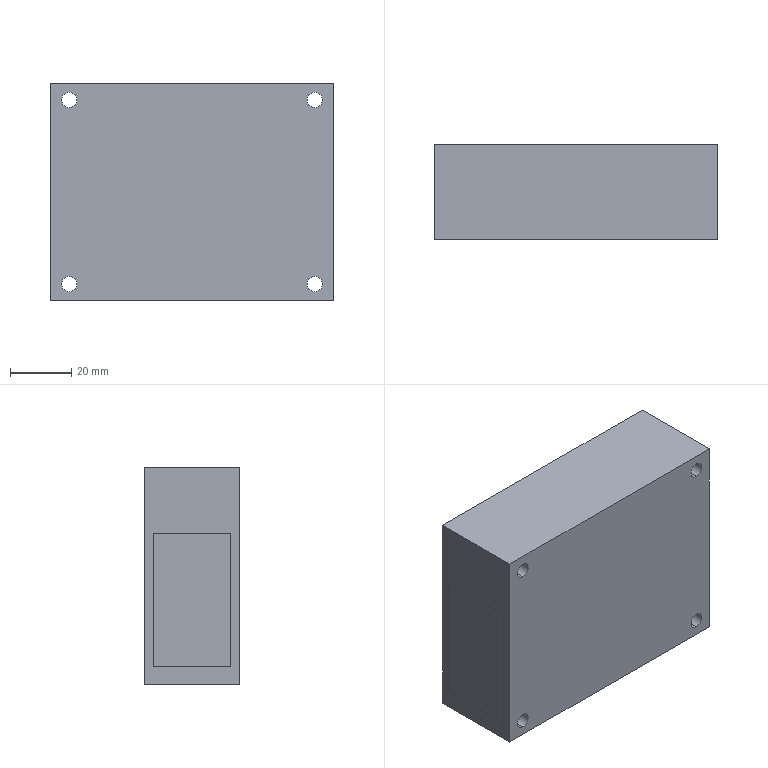Part | STEP file | Laser ranging sensor 1200mm | 1 solid | 19 faces | box 92 x 31 x 71 mm | volume 199839 mm3 | plane 11 | cylinder 8 | commonest cylinder face diameters 5 x8
STEP:
#1=CARTESIAN_POINT('',(-40.,15.5,-32.5));
#2=VERTEX_POINT('',#1);
#3=CARTESIAN_POINT('',(-40.,15.5,-27.5));
#4=VERTEX_POINT('',#3);
#5=CARTESIAN_POINT('',(-40.,15.5,-30.));
#6=DIRECTION('',(0.,1.,0.));
#7=DIRECTION('',(0.,0.,1.));
#8=AXIS2_PLACEMENT_3D('',#5,#6,#7);
#9=CIRCLE('',#8,2.5);
#10=EDGE_CURVE('',#2,#4,#9,.T.);
#11=ORIENTED_EDGE('',*,*,#10,.T.);
#12=CARTESIAN_POINT('',(-40.,-15.5,-27.5));
#13=VERTEX_POINT('',#12);
#14=CARTESIAN_POINT('',(-40.,15.5,-27.5));
#15=DIRECTION('',(0.,-1.,0.));
#16=VECTOR('',#15,1000.);
#17=LINE('',#14,#16);
#18=EDGE_CURVE('',#4,#13,#17,.T.);
#19=ORIENTED_EDGE('',*,*,#18,.T.);
#20=CARTESIAN_POINT('',(-40.,-15.5,-32.5));
#21=VERTEX_POINT('',#20);
#22=CARTESIAN_POINT('',(-40.,-15.5,-30.));
#23=DIRECTION('',(0.,1.,0.));
#24=DIRECTION('',(0.,0.,1.));
#25=AXIS2_PLACEMENT_3D('',#22,#23,#24);
#26=CIRCLE('',#25,2.5);
#27=EDGE_CURVE('',#21,#13,#26,.T.);
#28=ORIENTED_EDGE('',*,*,#27,.F.);
#29=CARTESIAN_POINT('',(-40.,15.5,-32.5));
#30=DIRECTION('',(0.,-1.,0.));
#31=VECTOR('',#30,1000.);
#32=LINE('',#29,#31);
#33=EDGE_CURVE('',#2,#21,#32,.T.);
#34=ORIENTED_EDGE('',*,*,#33,.F.);
#35=EDGE_LOOP('',(#11,#19,#28,#34));
#36=FACE_OUTER_BOUND('',#35,.T.);
#37=CARTESIAN_POINT('',(-40.,15.5,-30.));
#38=DIRECTION('',(0.,-1.,0.));
#39=DIRECTION('',(0.,0.,-1.));
#40=AXIS2_PLACEMENT_3D('',#37,#38,#39);
#41=CYLINDRICAL_SURFACE('',#40,2.5);
#42=ADVANCED_FACE('',(#36),#41,.F.);
#43=CARTESIAN_POINT('',(40.,15.5,-32.5));
#44=VERTEX_POINT('',#43);
#45=CARTESIAN_POINT('',(40.,15.5,-27.5));
#46=VERTEX_POINT('',#45);
#47=CARTESIAN_POINT('',(40.,15.5,-30.));
#48=DIRECTION('',(0.,1.,0.));
#49=DIRECTION('',(0.,0.,1.));
#50=AXIS2_PLACEMENT_3D('',#47,#48,#49);
#51=CIRCLE('',#50,2.5);
#52=EDGE_CURVE('',#44,#46,#51,.T.);
#53=ORIENTED_EDGE('',*,*,#52,.T.);
#54=CARTESIAN_POINT('',(40.,-15.5,-27.5));
#55=VERTEX_POINT('',#54);
#56=CARTESIAN_POINT('',(40.,15.5,-27.5));
#57=DIRECTION('',(0.,-1.,0.));
#58=VECTOR('',#57,1000.);
#59=LINE('',#56,#58);
#60=EDGE_CURVE('',#46,#55,#59,.T.);
#61=ORIENTED_EDGE('',*,*,#60,.T.);
#62=CARTESIAN_POINT('',(40.,-15.5,-32.5));
#63=VERTEX_POINT('',#62);
#64=CARTESIAN_POINT('',(40.,-15.5,-30.));
#65=DIRECTION('',(0.,1.,0.));
#66=DIRECTION('',(0.,0.,1.));
#67=AXIS2_PLACEMENT_3D('',#64,#65,#66);
#68=CIRCLE('',#67,2.5);
#69=EDGE_CURVE('',#63,#55,#68,.T.);
#70=ORIENTED_EDGE('',*,*,#69,.F.);
#71=CARTESIAN_POINT('',(40.,15.5,-32.5));
#72=DIRECTION('',(0.,-1.,0.));
#73=VECTOR('',#72,1000.);
#74=LINE('',#71,#73);
#75=EDGE_CURVE('',#44,#63,#74,.T.);
#76=ORIENTED_EDGE('',*,*,#75,.F.);
#77=EDGE_LOOP('',(#53,#61,#70,#76));
#78=FACE_OUTER_BOUND('',#77,.T.);
#79=CARTESIAN_POINT('',(40.,15.5,-30.));
#80=DIRECTION('',(0.,-1.,0.));
#81=DIRECTION('',(0.,0.,-1.));
#82=AXIS2_PLACEMENT_3D('',#79,#80,#81);
#83=CYLINDRICAL_SURFACE('',#82,2.5);
#84=ADVANCED_FACE('',(#78),#83,.F.);
#85=CARTESIAN_POINT('',(40.,15.5,27.5));
#86=VERTEX_POINT('',#85);
#87=CARTESIAN_POINT('',(40.,15.5,32.5));
#88=VERTEX_POINT('',#87);
#89=CARTESIAN_POINT('',(40.,15.5,30.));
#90=DIRECTION('',(0.,1.,0.));
#91=DIRECTION('',(0.,0.,1.));
#92=AXIS2_PLACEMENT_3D('',#89,#90,#91);
#93=CIRCLE('',#92,2.5);
#94=EDGE_CURVE('',#86,#88,#93,.T.);
#95=ORIENTED_EDGE('',*,*,#94,.T.);
#96=CARTESIAN_POINT('',(40.,-15.5,32.5));
#97=VERTEX_POINT('',#96);
#98=CARTESIAN_POINT('',(40.,15.5,32.5));
#99=DIRECTION('',(0.,-1.,0.));
#100=VECTOR('',#99,1000.);
#101=LINE('',#98,#100);
#102=EDGE_CURVE('',#88,#97,#101,.T.);
#103=ORIENTED_EDGE('',*,*,#102,.T.);
#104=CARTESIAN_POINT('',(40.,-15.5,27.5));
#105=VERTEX_POINT('',#104);
#106=CARTESIAN_POINT('',(40.,-15.5,30.));
#107=DIRECTION('',(0.,1.,0.));
#108=DIRECTION('',(0.,0.,1.));
#109=AXIS2_PLACEMENT_3D('',#106,#107,#108);
#110=CIRCLE('',#109,2.5);
#111=EDGE_CURVE('',#105,#97,#110,.T.);
#112=ORIENTED_EDGE('',*,*,#111,.F.);
#113=CARTESIAN_POINT('',(40.,15.5,27.5));
#114=DIRECTION('',(0.,-1.,0.));
#115=VECTOR('',#114,1000.);
#116=LINE('',#113,#115);
#117=EDGE_CURVE('',#86,#105,#116,.T.);
#118=ORIENTED_EDGE('',*,*,#117,.F.);
#119=EDGE_LOOP('',(#95,#103,#112,#118));
#120=FACE_OUTER_BOUND('',#119,.T.);
#121=CARTESIAN_POINT('',(40.,15.5,30.));
#122=DIRECTION('',(0.,-1.,0.));
#123=DIRECTION('',(0.,0.,-1.));
#124=AXIS2_PLACEMENT_3D('',#121,#122,#123);
#125=CYLINDRICAL_SURFACE('',#124,2.5);
#126=ADVANCED_FACE('',(#120),#125,.F.);
#127=CARTESIAN_POINT('',(-40.,15.5,27.5));
#128=VERTEX_POINT('',#127);
#129=CARTESIAN_POINT('',(-40.,15.5,32.5));
#130=VERTEX_POINT('',#129);
#131=CARTESIAN_POINT('',(-40.,15.5,30.));
#132=DIRECTION('',(0.,1.,0.));
#133=DIRECTION('',(0.,0.,1.));
#134=AXIS2_PLACEMENT_3D('',#131,#132,#133);
#135=CIRCLE('',#134,2.5);
#136=EDGE_CURVE('',#128,#130,#135,.T.);
#137=ORIENTED_EDGE('',*,*,#136,.T.);
#138=CARTESIAN_POINT('',(-40.,-15.5,32.5));
#139=VERTEX_POINT('',#138);
#140=CARTESIAN_POINT('',(-40.,15.5,32.5));
#141=DIRECTION('',(0.,-1.,0.));
#142=VECTOR('',#141,1000.);
#143=LINE('',#140,#142);
#144=EDGE_CURVE('',#130,#139,#143,.T.);
#145=ORIENTED_EDGE('',*,*,#144,.T.);
#146=CARTESIAN_POINT('',(-40.,-15.5,27.5));
#147=VERTEX_POINT('',#146);
#148=CARTESIAN_POINT('',(-40.,-15.5,30.));
#149=DIRECTION('',(0.,1.,0.));
#150=DIRECTION('',(0.,0.,1.));
#151=AXIS2_PLACEMENT_3D('',#148,#149,#150);
#152=CIRCLE('',#151,2.5);
#153=EDGE_CURVE('',#147,#139,#152,.T.);
#154=ORIENTED_EDGE('',*,*,#153,.F.);
#155=CARTESIAN_POINT('',(-40.,15.5,27.5));
#156=DIRECTION('',(0.,-1.,0.));
#157=VECTOR('',#156,1000.);
#158=LINE('',#155,#157);
#159=EDGE_CURVE('',#128,#147,#158,.T.);
#160=ORIENTED_EDGE('',*,*,#159,.F.);
#161=EDGE_LOOP('',(#137,#145,#154,#160));
#162=FACE_OUTER_BOUND('',#161,.T.);
#163=CARTESIAN_POINT('',(-40.,15.5,30.));
#164=DIRECTION('',(0.,-1.,0.));
#165=DIRECTION('',(0.,0.,-1.));
#166=AXIS2_PLACEMENT_3D('',#163,#164,#165);
#167=CYLINDRICAL_SURFACE('',#166,2.5);
#168=ADVANCED_FACE('',(#162),#167,.F.);
#169=CARTESIAN_POINT('',(46.,15.5,35.5));
#170=VERTEX_POINT('',#169);
#171=CARTESIAN_POINT('',(46.,15.5,-35.5));
#172=VERTEX_POINT('',#171);
#173=CARTESIAN_POINT('',(46.,15.5,35.5));
#174=DIRECTION('',(0.,0.,-1.));
#175=VECTOR('',#174,1000.);
#176=LINE('',#173,#175);
#177=EDGE_CURVE('',#170,#172,#176,.T.);
#178=ORIENTED_EDGE('',*,*,#177,.T.);
#179=CARTESIAN_POINT('',(-46.,15.5,-35.5));
#180=VERTEX_POINT('',#179);
#181=CARTESIAN_POINT('',(-46.,15.5,-35.5));
#182=DIRECTION('',(-1.,0.,0.));
#183=VECTOR('',#182,1000.);
#184=LINE('',#181,#183);
#185=EDGE_CURVE('',#172,#180,#184,.T.);
#186=ORIENTED_EDGE('',*,*,#185,.T.);
#187=CARTESIAN_POINT('',(-46.,15.5,35.5));
#188=VERTEX_POINT('',#187);
#189=CARTESIAN_POINT('',(-46.,15.5,35.5));
#190=DIRECTION('',(0.,0.,1.));
#191=VECTOR('',#190,1000.);
#192=LINE('',#189,#191);
#193=EDGE_CURVE('',#180,#188,#192,.T.);
#194=ORIENTED_EDGE('',*,*,#193,.T.);
#195=CARTESIAN_POINT('',(-46.,15.5,35.5));
#196=DIRECTION('',(1.,0.,0.));
#197=VECTOR('',#196,1000.);
#198=LINE('',#195,#197);
#199=EDGE_CURVE('',#188,#170,#198,.T.);
#200=ORIENTED_EDGE('',*,*,#199,.T.);
#201=EDGE_LOOP('',(#178,#186,#194,#200));
#202=FACE_OUTER_BOUND('',#201,.T.);
#203=ORIENTED_EDGE('',*,*,#136,.F.);
#204=CARTESIAN_POINT('',(-40.,15.5,30.));
#205=DIRECTION('',(0.,1.,0.));
#206=DIRECTION('',(0.,0.,1.));
#207=AXIS2_PLACEMENT_3D('',#204,#205,#206);
#208=CIRCLE('',#207,2.5);
#209=EDGE_CURVE('',#130,#128,#208,.T.);
#210=ORIENTED_EDGE('',*,*,#209,.F.);
#211=EDGE_LOOP('',(#203,#210));
#212=FACE_BOUND('',#211,.T.);
#213=ORIENTED_EDGE('',*,*,#94,.F.);
#214=CARTESIAN_POINT('',(40.,15.5,30.));
#215=DIRECTION('',(0.,1.,0.));
#216=DIRECTION('',(0.,0.,1.));
#217=AXIS2_PLACEMENT_3D('',#214,#215,#216);
#218=CIRCLE('',#217,2.5);
#219=EDGE_CURVE('',#88,#86,#218,.T.);
#220=ORIENTED_EDGE('',*,*,#219,.F.);
#221=EDGE_LOOP('',(#213,#220));
#222=FACE_BOUND('',#221,.T.);
#223=ORIENTED_EDGE('',*,*,#52,.F.);
#224=CARTESIAN_POINT('',(40.,15.5,-30.));
#225=DIRECTION('',(0.,1.,0.));
#226=DIRECTION('',(0.,0.,1.));
#227=AXIS2_PLACEMENT_3D('',#224,#225,#226);
#228=CIRCLE('',#227,2.5);
#229=EDGE_CURVE('',#46,#44,#228,.T.);
#230=ORIENTED_EDGE('',*,*,#229,.F.);
#231=EDGE_LOOP('',(#223,#230));
#232=FACE_BOUND('',#231,.T.);
#233=ORIENTED_EDGE('',*,*,#10,.F.);
#234=CARTESIAN_POINT('',(-40.,15.5,-30.));
#235=DIRECTION('',(0.,1.,0.));
#236=DIRECTION('',(0.,0.,1.));
#237=AXIS2_PLACEMENT_3D('',#234,#235,#236);
#238=CIRCLE('',#237,2.5);
#239=EDGE_CURVE('',#4,#2,#238,.T.);
#240=ORIENTED_EDGE('',*,*,#239,.F.);
#241=EDGE_LOOP('',(#233,#240));
#242=FACE_BOUND('',#241,.T.);
#243=CARTESIAN_POINT('',(0.,15.5,0.));
#244=DIRECTION('',(0.,-1.,0.));
#245=DIRECTION('',(0.,0.,-1.));
#246=AXIS2_PLACEMENT_3D('',#243,#244,#245);
#247=PLANE('',#246);
#248=ADVANCED_FACE('',(#202,#212,#222,#232,#242),#247,.F.);
#249=ORIENTED_EDGE('',*,*,#69,.T.);
#250=CARTESIAN_POINT('',(40.,-15.5,-30.));
#251=DIRECTION('',(0.,1.,0.));
#252=DIRECTION('',(0.,0.,1.));
#253=AXIS2_PLACEMENT_3D('',#250,#251,#252);
#254=CIRCLE('',#253,2.5);
#255=EDGE_CURVE('',#55,#63,#254,.T.);
#256=ORIENTED_EDGE('',*,*,#255,.T.);
#257=EDGE_LOOP('',(#249,#256));
#258=FACE_BOUND('',#257,.T.);
#259=ORIENTED_EDGE('',*,*,#153,.T.);
#260=CARTESIAN_POINT('',(-40.,-15.5,30.));
#261=DIRECTION('',(0.,1.,0.));
#262=DIRECTION('',(0.,0.,1.));
#263=AXIS2_PLACEMENT_3D('',#260,#261,#262);
#264=CIRCLE('',#263,2.5);
#265=EDGE_CURVE('',#139,#147,#264,.T.);
#266=ORIENTED_EDGE('',*,*,#265,.T.);
#267=EDGE_LOOP('',(#259,#266));
#268=FACE_BOUND('',#267,.T.);
#269=CARTESIAN_POINT('',(46.,-15.5,35.5));
#270=VERTEX_POINT('',#269);
#271=CARTESIAN_POINT('',(46.,-15.5,-35.5));
#272=VERTEX_POINT('',#271);
#273=CARTESIAN_POINT('',(46.,-15.5,35.5));
#274=DIRECTION('',(0.,0.,-1.));
#275=VECTOR('',#274,1000.);
#276=LINE('',#273,#275);
#277=EDGE_CURVE('',#270,#272,#276,.T.);
#278=ORIENTED_EDGE('',*,*,#277,.F.);
#279=CARTESIAN_POINT('',(-46.,-15.5,35.5));
#280=VERTEX_POINT('',#279);
#281=CARTESIAN_POINT('',(-46.,-15.5,35.5));
#282=DIRECTION('',(1.,0.,0.));
#283=VECTOR('',#282,1000.);
#284=LINE('',#281,#283);
#285=EDGE_CURVE('',#280,#270,#284,.T.);
#286=ORIENTED_EDGE('',*,*,#285,.F.);
#287=CARTESIAN_POINT('',(-46.,-15.5,-35.5));
#288=VERTEX_POINT('',#287);
#289=CARTESIAN_POINT('',(-46.,-15.5,35.5));
#290=DIRECTION('',(0.,0.,1.));
#291=VECTOR('',#290,1000.);
#292=LINE('',#289,#291);
#293=EDGE_CURVE('',#288,#280,#292,.T.);
#294=ORIENTED_EDGE('',*,*,#293,.F.);
#295=CARTESIAN_POINT('',(-46.,-15.5,-35.5));
#296=DIRECTION('',(-1.,0.,0.));
#297=VECTOR('',#296,1000.);
#298=LINE('',#295,#297);
#299=EDGE_CURVE('',#272,#288,#298,.T.);
#300=ORIENTED_EDGE('',*,*,#299,.F.);
#301=EDGE_LOOP('',(#278,#286,#294,#300));
#302=FACE_OUTER_BOUND('',#301,.T.);
#303=ORIENTED_EDGE('',*,*,#111,.T.);
#304=CARTESIAN_POINT('',(40.,-15.5,30.));
#305=DIRECTION('',(0.,1.,0.));
#306=DIRECTION('',(0.,0.,1.));
#307=AXIS2_PLACEMENT_3D('',#304,#305,#306);
#308=CIRCLE('',#307,2.5);
#309=EDGE_CURVE('',#97,#105,#308,.T.);
#310=ORIENTED_EDGE('',*,*,#309,.T.);
#311=EDGE_LOOP('',(#303,#310));
#312=FACE_BOUND('',#311,.T.);
#313=ORIENTED_EDGE('',*,*,#27,.T.);
#314=CARTESIAN_POINT('',(-40.,-15.5,-30.));
#315=DIRECTION('',(0.,1.,0.));
#316=DIRECTION('',(0.,0.,1.));
#317=AXIS2_PLACEMENT_3D('',#314,#315,#316);
#318=CIRCLE('',#317,2.5);
#319=EDGE_CURVE('',#13,#21,#318,.T.);
#320=ORIENTED_EDGE('',*,*,#319,.T.);
#321=EDGE_LOOP('',(#313,#320));
#322=FACE_BOUND('',#321,.T.);
#323=CARTESIAN_POINT('',(0.,-15.5,0.));
#324=DIRECTION('',(0.,-1.,0.));
#325=DIRECTION('',(0.,0.,-1.));
#326=AXIS2_PLACEMENT_3D('',#323,#324,#325);
#327=PLANE('',#326);
#328=ADVANCED_FACE('',(#258,#268,#302,#312,#322),#327,.T.);
#329=ORIENTED_EDGE('',*,*,#277,.T.);
#330=CARTESIAN_POINT('',(46.,15.5,-35.5));
#331=DIRECTION('',(0.,-1.,0.));
#332=VECTOR('',#331,1000.);
#333=LINE('',#330,#332);
#334=EDGE_CURVE('',#172,#272,#333,.T.);
#335=ORIENTED_EDGE('',*,*,#334,.F.);
#336=ORIENTED_EDGE('',*,*,#177,.F.);
#337=CARTESIAN_POINT('',(46.,15.5,35.5));
#338=DIRECTION('',(0.,-1.,0.));
#339=VECTOR('',#338,1000.);
#340=LINE('',#337,#339);
#341=EDGE_CURVE('',#170,#270,#340,.T.);
#342=ORIENTED_EDGE('',*,*,#341,.T.);
#343=EDGE_LOOP('',(#329,#335,#336,#342));
#344=FACE_OUTER_BOUND('',#343,.T.);
#345=CARTESIAN_POINT('',(46.,15.5,35.5));
#346=DIRECTION('',(-1.,0.,0.));
#347=DIRECTION('',(0.,0.,1.));
#348=AXIS2_PLACEMENT_3D('',#345,#346,#347);
#349=PLANE('',#348);
#350=ADVANCED_FACE('',(#344),#349,.F.);
#351=ORIENTED_EDGE('',*,*,#299,.T.);
#352=CARTESIAN_POINT('',(-46.,15.5,-35.5));
#353=DIRECTION('',(0.,-1.,0.));
#354=VECTOR('',#353,1000.);
#355=LINE('',#352,#354);
#356=EDGE_CURVE('',#180,#288,#355,.T.);
#357=ORIENTED_EDGE('',*,*,#356,.F.);
#358=ORIENTED_EDGE('',*,*,#185,.F.);
#359=ORIENTED_EDGE('',*,*,#334,.T.);
#360=EDGE_LOOP('',(#351,#357,#358,#359));
#361=FACE_OUTER_BOUND('',#360,.T.);
#362=CARTESIAN_POINT('',(-46.,15.5,-35.5));
#363=DIRECTION('',(0.,0.,1.));
#364=DIRECTION('',(1.,0.,0.));
#365=AXIS2_PLACEMENT_3D('',#362,#363,#364);
#366=PLANE('',#365);
#367=ADVANCED_FACE('',(#361),#366,.F.);
#368=CARTESIAN_POINT('',(-46.,12.595,13.805));
#369=VERTEX_POINT('',#368);
#370=CARTESIAN_POINT('',(-46.,12.595,-29.542));
#371=VERTEX_POINT('',#370);
#372=CARTESIAN_POINT('',(-46.,12.595,-29.542));
#373=DIRECTION('',(0.,0.,-1.));
#374=VECTOR('',#373,1000.);
#375=LINE('',#372,#374);
#376=EDGE_CURVE('',#369,#371,#375,.T.);
#377=ORIENTED_EDGE('',*,*,#376,.F.);
#378=CARTESIAN_POINT('',(-46.,-12.595,13.805));
#379=VERTEX_POINT('',#378);
#380=CARTESIAN_POINT('',(-46.,-12.595,13.805));
#381=DIRECTION('',(0.,1.,0.));
#382=VECTOR('',#381,1000.);
#383=LINE('',#380,#382);
#384=EDGE_CURVE('',#379,#369,#383,.T.);
#385=ORIENTED_EDGE('',*,*,#384,.F.);
#386=CARTESIAN_POINT('',(-46.,-12.595,-29.542));
#387=VERTEX_POINT('',#386);
#388=CARTESIAN_POINT('',(-46.,-12.595,-29.542));
#389=DIRECTION('',(0.,0.,1.));
#390=VECTOR('',#389,1000.);
#391=LINE('',#388,#390);
#392=EDGE_CURVE('',#387,#379,#391,.T.);
#393=ORIENTED_EDGE('',*,*,#392,.F.);
#394=CARTESIAN_POINT('',(-46.,-12.595,-29.542));
#395=DIRECTION('',(0.,-1.,0.));
#396=VECTOR('',#395,1000.);
#397=LINE('',#394,#396);
#398=EDGE_CURVE('',#371,#387,#397,.T.);
#399=ORIENTED_EDGE('',*,*,#398,.F.);
#400=EDGE_LOOP('',(#377,#385,#393,#399));
#401=FACE_BOUND('',#400,.T.);
#402=ORIENTED_EDGE('',*,*,#293,.T.);
#403=CARTESIAN_POINT('',(-46.,15.5,35.5));
#404=DIRECTION('',(0.,-1.,0.));
#405=VECTOR('',#404,1000.);
#406=LINE('',#403,#405);
#407=EDGE_CURVE('',#188,#280,#406,.T.);
#408=ORIENTED_EDGE('',*,*,#407,.F.);
#409=ORIENTED_EDGE('',*,*,#193,.F.);
#410=ORIENTED_EDGE('',*,*,#356,.T.);
#411=EDGE_LOOP('',(#402,#408,#409,#410));
#412=FACE_OUTER_BOUND('',#411,.T.);
#413=CARTESIAN_POINT('',(-46.,15.5,35.5));
#414=DIRECTION('',(1.,0.,0.));
#415=DIRECTION('',(0.,0.,-1.));
#416=AXIS2_PLACEMENT_3D('',#413,#414,#415);
#417=PLANE('',#416);
#418=ADVANCED_FACE('',(#401,#412),#417,.F.);
#419=ORIENTED_EDGE('',*,*,#285,.T.);
#420=ORIENTED_EDGE('',*,*,#341,.F.);
#421=ORIENTED_EDGE('',*,*,#199,.F.);
#422=ORIENTED_EDGE('',*,*,#407,.T.);
#423=EDGE_LOOP('',(#419,#420,#421,#422));
#424=FACE_OUTER_BOUND('',#423,.T.);
#425=CARTESIAN_POINT('',(-46.,15.5,35.5));
#426=DIRECTION('',(0.,0.,-1.));
#427=DIRECTION('',(-1.,0.,0.));
#428=AXIS2_PLACEMENT_3D('',#425,#426,#427);
#429=PLANE('',#428);
#430=ADVANCED_FACE('',(#424),#429,.F.);
#431=ORIENTED_EDGE('',*,*,#144,.F.);
#432=ORIENTED_EDGE('',*,*,#209,.T.);
#433=ORIENTED_EDGE('',*,*,#159,.T.);
#434=ORIENTED_EDGE('',*,*,#265,.F.);
#435=EDGE_LOOP('',(#431,#432,#433,#434));
#436=FACE_OUTER_BOUND('',#435,.T.);
#437=CARTESIAN_POINT('',(-40.,15.5,30.));
#438=DIRECTION('',(0.,-1.,0.));
#439=DIRECTION('',(0.,0.,-1.));
#440=AXIS2_PLACEMENT_3D('',#437,#438,#439);
#441=CYLINDRICAL_SURFACE('',#440,2.5);
#442=ADVANCED_FACE('',(#436),#441,.F.);
#443=ORIENTED_EDGE('',*,*,#102,.F.);
#444=ORIENTED_EDGE('',*,*,#219,.T.);
#445=ORIENTED_EDGE('',*,*,#117,.T.);
#446=ORIENTED_EDGE('',*,*,#309,.F.);
#447=EDGE_LOOP('',(#443,#444,#445,#446));
#448=FACE_OUTER_BOUND('',#447,.T.);
#449=CARTESIAN_POINT('',(40.,15.5,30.));
#450=DIRECTION('',(0.,-1.,0.));
#451=DIRECTION('',(0.,0.,-1.));
#452=AXIS2_PLACEMENT_3D('',#449,#450,#451);
#453=CYLINDRICAL_SURFACE('',#452,2.5);
#454=ADVANCED_FACE('',(#448),#453,.F.);
#455=ORIENTED_EDGE('',*,*,#60,.F.);
#456=ORIENTED_EDGE('',*,*,#229,.T.);
#457=ORIENTED_EDGE('',*,*,#75,.T.);
#458=ORIENTED_EDGE('',*,*,#255,.F.);
#459=EDGE_LOOP('',(#455,#456,#457,#458));
#460=FACE_OUTER_BOUND('',#459,.T.);
#461=CARTESIAN_POINT('',(40.,15.5,-30.));
#462=DIRECTION('',(0.,-1.,0.));
#463=DIRECTION('',(0.,0.,-1.));
#464=AXIS2_PLACEMENT_3D('',#461,#462,#463);
#465=CYLINDRICAL_SURFACE('',#464,2.5);
#466=ADVANCED_FACE('',(#460),#465,.F.);
#467=ORIENTED_EDGE('',*,*,#18,.F.);
#468=ORIENTED_EDGE('',*,*,#239,.T.);
#469=ORIENTED_EDGE('',*,*,#33,.T.);
#470=ORIENTED_EDGE('',*,*,#319,.F.);
#471=EDGE_LOOP('',(#467,#468,#469,#470));
#472=FACE_OUTER_BOUND('',#471,.T.);
#473=CARTESIAN_POINT('',(-40.,15.5,-30.));
#474=DIRECTION('',(0.,-1.,0.));
#475=DIRECTION('',(0.,0.,-1.));
#476=AXIS2_PLACEMENT_3D('',#473,#474,#475);
#477=CYLINDRICAL_SURFACE('',#476,2.5);
#478=ADVANCED_FACE('',(#472),#477,.F.);
#479=ORIENTED_EDGE('',*,*,#384,.T.);
#480=CARTESIAN_POINT('',(-45.8,12.595,13.805));
#481=VERTEX_POINT('',#480);
#482=CARTESIAN_POINT('',(-45.8,12.595,13.805));
#483=DIRECTION('',(-1.,0.,0.));
#484=VECTOR('',#483,1000.);
#485=LINE('',#482,#484);
#486=EDGE_CURVE('',#481,#369,#485,.T.);
#487=ORIENTED_EDGE('',*,*,#486,.F.);
#488=CARTESIAN_POINT('',(-45.8,-12.595,13.805));
#489=VERTEX_POINT('',#488);
#490=CARTESIAN_POINT('',(-45.8,-12.595,13.805));
#491=DIRECTION('',(0.,1.,0.));
#492=VECTOR('',#491,1000.);
#493=LINE('',#490,#492);
#494=EDGE_CURVE('',#489,#481,#493,.T.);
#495=ORIENTED_EDGE('',*,*,#494,.F.);
#496=CARTESIAN_POINT('',(-45.8,-12.595,13.805));
#497=DIRECTION('',(-1.,0.,0.));
#498=VECTOR('',#497,1000.);
#499=LINE('',#496,#498);
#500=EDGE_CURVE('',#489,#379,#499,.T.);
#501=ORIENTED_EDGE('',*,*,#500,.T.);
#502=EDGE_LOOP('',(#479,#487,#495,#501));
#503=FACE_OUTER_BOUND('',#502,.T.);
#504=CARTESIAN_POINT('',(-45.8,-12.595,13.805));
#505=DIRECTION('',(0.,0.,1.));
#506=DIRECTION('',(1.,0.,0.));
#507=AXIS2_PLACEMENT_3D('',#504,#505,#506);
#508=PLANE('',#507);
#509=ADVANCED_FACE('',(#503),#508,.F.);
#510=ORIENTED_EDGE('',*,*,#392,.T.);
#511=ORIENTED_EDGE('',*,*,#500,.F.);
#512=CARTESIAN_POINT('',(-45.8,-12.595,-29.542));
#513=VERTEX_POINT('',#512);
#514=CARTESIAN_POINT('',(-45.8,-12.595,-29.542));
#515=DIRECTION('',(0.,0.,1.));
#516=VECTOR('',#515,1000.);
#517=LINE('',#514,#516);
#518=EDGE_CURVE('',#513,#489,#517,.T.);
#519=ORIENTED_EDGE('',*,*,#518,.F.);
#520=CARTESIAN_POINT('',(-45.8,-12.595,-29.542));
#521=DIRECTION('',(-1.,0.,0.));
#522=VECTOR('',#521,1000.);
#523=LINE('',#520,#522);
#524=EDGE_CURVE('',#513,#387,#523,.T.);
#525=ORIENTED_EDGE('',*,*,#524,.T.);
#526=EDGE_LOOP('',(#510,#511,#519,#525));
#527=FACE_OUTER_BOUND('',#526,.T.);
#528=CARTESIAN_POINT('',(-45.8,-12.595,-29.542));
#529=DIRECTION('',(0.,-1.,0.));
#530=DIRECTION('',(0.,0.,-1.));
#531=AXIS2_PLACEMENT_3D('',#528,#529,#530);
#532=PLANE('',#531);
#533=ADVANCED_FACE('',(#527),#532,.F.);
#534=ORIENTED_EDGE('',*,*,#398,.T.);
#535=ORIENTED_EDGE('',*,*,#524,.F.);
#536=CARTESIAN_POINT('',(-45.8,12.595,-29.542));
#537=VERTEX_POINT('',#536);
#538=CARTESIAN_POINT('',(-45.8,-12.595,-29.542));
#539=DIRECTION('',(0.,-1.,0.));
#540=VECTOR('',#539,1000.);
#541=LINE('',#538,#540);
#542=EDGE_CURVE('',#537,#513,#541,.T.);
#543=ORIENTED_EDGE('',*,*,#542,.F.);
#544=CARTESIAN_POINT('',(-45.8,12.595,-29.542));
#545=DIRECTION('',(-1.,0.,0.));
#546=VECTOR('',#545,1000.);
#547=LINE('',#544,#546);
#548=EDGE_CURVE('',#537,#371,#547,.T.);
#549=ORIENTED_EDGE('',*,*,#548,.T.);
#550=EDGE_LOOP('',(#534,#535,#543,#549));
#551=FACE_OUTER_BOUND('',#550,.T.);
#552=CARTESIAN_POINT('',(-45.8,-12.595,-29.542));
#553=DIRECTION('',(0.,0.,-1.));
#554=DIRECTION('',(-1.,0.,0.));
#555=AXIS2_PLACEMENT_3D('',#552,#553,#554);
#556=PLANE('',#555);
#557=ADVANCED_FACE('',(#551),#556,.F.);
#558=ORIENTED_EDGE('',*,*,#376,.T.);
#559=ORIENTED_EDGE('',*,*,#548,.F.);
#560=CARTESIAN_POINT('',(-45.8,12.595,-29.542));
#561=DIRECTION('',(0.,0.,-1.));
#562=VECTOR('',#561,1000.);
#563=LINE('',#560,#562);
#564=EDGE_CURVE('',#481,#537,#563,.T.);
#565=ORIENTED_EDGE('',*,*,#564,.F.);
#566=ORIENTED_EDGE('',*,*,#486,.T.);
#567=EDGE_LOOP('',(#558,#559,#565,#566));
#568=FACE_OUTER_BOUND('',#567,.T.);
#569=CARTESIAN_POINT('',(-45.8,12.595,-29.542));
#570=DIRECTION('',(0.,1.,0.));
#571=DIRECTION('',(0.,0.,1.));
#572=AXIS2_PLACEMENT_3D('',#569,#570,#571);
#573=PLANE('',#572);
#574=ADVANCED_FACE('',(#568),#573,.F.);
#575=ORIENTED_EDGE('',*,*,#494,.T.);
#576=ORIENTED_EDGE('',*,*,#564,.T.);
#577=ORIENTED_EDGE('',*,*,#542,.T.);
#578=ORIENTED_EDGE('',*,*,#518,.T.);
#579=EDGE_LOOP('',(#575,#576,#577,#578));
#580=FACE_OUTER_BOUND('',#579,.T.);
#581=CARTESIAN_POINT('',(-45.8,0.,0.));
#582=DIRECTION('',(1.,0.,0.));
#583=DIRECTION('',(0.,0.,-1.));
#584=AXIS2_PLACEMENT_3D('',#581,#582,#583);
#585=PLANE('',#584);
#586=ADVANCED_FACE('',(#580),#585,.F.);
#587=CLOSED_SHELL('',(#42,#84,#126,#168,#248,#328,#350,#367,#418,#430,#442,#454,#466,#478,#509,#533,#557,#574,#586));
#588=MANIFOLD_SOLID_BREP('',#587);
#589=CARTESIAN_POINT('',(0.,0.,0.));
#590=DIRECTION('',(0.,0.,1.));
#591=DIRECTION('',(1.,0.,0.));
#592=AXIS2_PLACEMENT_3D('',#589,#590,#591);
#593=(LENGTH_UNIT()NAMED_UNIT(*)SI_UNIT(.MILLI.,.METRE.));
#594=UNCERTAINTY_MEASURE_WITH_UNIT(LENGTH_MEASURE(0.00001),#593,'','');
#595=(NAMED_UNIT(*)PLANE_ANGLE_UNIT()SI_UNIT($,.RADIAN.));
#596=(NAMED_UNIT(*)SI_UNIT($,.STERADIAN.)SOLID_ANGLE_UNIT());
#597=(GEOMETRIC_REPRESENTATION_CONTEXT(3)GLOBAL_UNCERTAINTY_ASSIGNED_CONTEXT((#594))GLOBAL_UNIT_ASSIGNED_CONTEXT((#593,#595,#596))REPRESENTATION_CONTEXT('',''));
#598=ADVANCED_BREP_SHAPE_REPRESENTATION('',(#588,#592),#597);